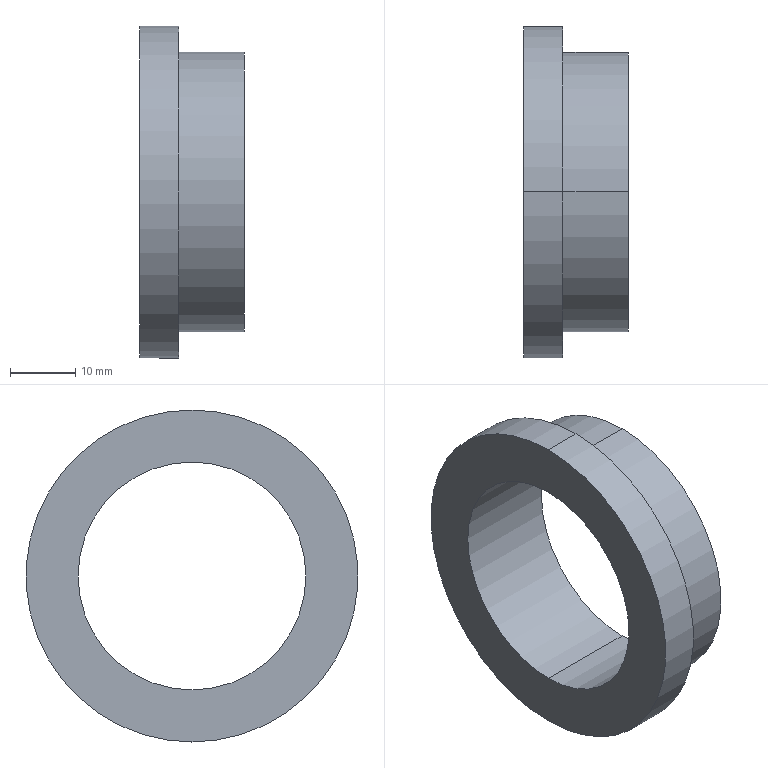Part | SolidWorks | features Revolution 1 | 1 solid | 9 faces | box 16 x 51 x 51 mm | volume 11385 mm3 | cylinder 6 | plane 3 | commonest cylinder face diameters 35 x2 43 x2 51 x2
STEP:
#1=CARTESIAN_POINT('',(-15.343,0.,25.5));
#2=VERTEX_POINT('',#1);
#3=CARTESIAN_POINT('',(-15.343,0.,-25.5));
#4=VERTEX_POINT('',#3);
#5=CARTESIAN_POINT('',(-15.343,0.,0.));
#6=DIRECTION('',(-1.,0.,0.));
#7=DIRECTION('',(0.,0.,1.));
#8=AXIS2_PLACEMENT_3D('',#5,#6,#7);
#9=CIRCLE('',#8,25.5);
#10=EDGE_CURVE('',#2,#4,#9,.T.);
#11=ORIENTED_EDGE('',*,*,#10,.T.);
#12=CARTESIAN_POINT('',(-21.343,0.,-25.5));
#13=VERTEX_POINT('',#12);
#14=CARTESIAN_POINT('',(0.,0.,-25.5));
#15=DIRECTION('',(-1.,0.,0.));
#16=VECTOR('',#15,1000.);
#17=LINE('',#14,#16);
#18=EDGE_CURVE('',#4,#13,#17,.T.);
#19=ORIENTED_EDGE('',*,*,#18,.T.);
#20=CARTESIAN_POINT('',(-21.343,0.,25.5));
#21=VERTEX_POINT('',#20);
#22=CARTESIAN_POINT('',(-21.343,0.,0.));
#23=DIRECTION('',(-1.,0.,0.));
#24=DIRECTION('',(0.,0.,1.));
#25=AXIS2_PLACEMENT_3D('',#22,#23,#24);
#26=CIRCLE('',#25,25.5);
#27=EDGE_CURVE('',#21,#13,#26,.T.);
#28=ORIENTED_EDGE('',*,*,#27,.F.);
#29=CARTESIAN_POINT('',(0.,0.,25.5));
#30=DIRECTION('',(-1.,0.,0.));
#31=VECTOR('',#30,1000.);
#32=LINE('',#29,#31);
#33=EDGE_CURVE('',#2,#21,#32,.T.);
#34=ORIENTED_EDGE('',*,*,#33,.F.);
#35=EDGE_LOOP('',(#11,#19,#28,#34));
#36=FACE_OUTER_BOUND('',#35,.T.);
#37=CARTESIAN_POINT('',(0.,0.,0.));
#38=DIRECTION('',(-1.,0.,0.));
#39=DIRECTION('',(0.,0.,1.));
#40=AXIS2_PLACEMENT_3D('',#37,#38,#39);
#41=CYLINDRICAL_SURFACE('',#40,25.5);
#42=ADVANCED_FACE('',(#36),#41,.T.);
#43=CARTESIAN_POINT('',(-5.343,0.,21.5));
#44=VERTEX_POINT('',#43);
#45=CARTESIAN_POINT('',(-5.343,0.,-21.5));
#46=VERTEX_POINT('',#45);
#47=CARTESIAN_POINT('',(-5.343,0.,0.));
#48=DIRECTION('',(-1.,0.,0.));
#49=DIRECTION('',(0.,0.,1.));
#50=AXIS2_PLACEMENT_3D('',#47,#48,#49);
#51=CIRCLE('',#50,21.5);
#52=EDGE_CURVE('',#44,#46,#51,.T.);
#53=ORIENTED_EDGE('',*,*,#52,.T.);
#54=CARTESIAN_POINT('',(-15.343,0.,-21.5));
#55=VERTEX_POINT('',#54);
#56=CARTESIAN_POINT('',(0.,0.,-21.5));
#57=DIRECTION('',(-1.,0.,0.));
#58=VECTOR('',#57,1000.);
#59=LINE('',#56,#58);
#60=EDGE_CURVE('',#46,#55,#59,.T.);
#61=ORIENTED_EDGE('',*,*,#60,.T.);
#62=CARTESIAN_POINT('',(-15.343,0.,21.5));
#63=VERTEX_POINT('',#62);
#64=CARTESIAN_POINT('',(-15.343,0.,0.));
#65=DIRECTION('',(-1.,0.,0.));
#66=DIRECTION('',(0.,0.,1.));
#67=AXIS2_PLACEMENT_3D('',#64,#65,#66);
#68=CIRCLE('',#67,21.5);
#69=EDGE_CURVE('',#63,#55,#68,.T.);
#70=ORIENTED_EDGE('',*,*,#69,.F.);
#71=CARTESIAN_POINT('',(0.,0.,21.5));
#72=DIRECTION('',(-1.,0.,0.));
#73=VECTOR('',#72,1000.);
#74=LINE('',#71,#73);
#75=EDGE_CURVE('',#44,#63,#74,.T.);
#76=ORIENTED_EDGE('',*,*,#75,.F.);
#77=EDGE_LOOP('',(#53,#61,#70,#76));
#78=FACE_OUTER_BOUND('',#77,.T.);
#79=CARTESIAN_POINT('',(0.,0.,0.));
#80=DIRECTION('',(-1.,0.,0.));
#81=DIRECTION('',(0.,0.,1.));
#82=AXIS2_PLACEMENT_3D('',#79,#80,#81);
#83=CYLINDRICAL_SURFACE('',#82,21.5);
#84=ADVANCED_FACE('',(#78),#83,.T.);
#85=CARTESIAN_POINT('',(-5.343,0.,-17.5));
#86=VERTEX_POINT('',#85);
#87=CARTESIAN_POINT('',(-5.343,0.,17.5));
#88=VERTEX_POINT('',#87);
#89=CARTESIAN_POINT('',(-5.343,0.,0.));
#90=DIRECTION('',(-1.,0.,0.));
#91=DIRECTION('',(0.,0.,1.));
#92=AXIS2_PLACEMENT_3D('',#89,#90,#91);
#93=CIRCLE('',#92,17.5);
#94=EDGE_CURVE('',#86,#88,#93,.T.);
#95=ORIENTED_EDGE('',*,*,#94,.F.);
#96=CARTESIAN_POINT('',(-21.343,0.,-17.5));
#97=VERTEX_POINT('',#96);
#98=CARTESIAN_POINT('',(0.,0.,-17.5));
#99=DIRECTION('',(-1.,0.,0.));
#100=VECTOR('',#99,1000.);
#101=LINE('',#98,#100);
#102=EDGE_CURVE('',#86,#97,#101,.T.);
#103=ORIENTED_EDGE('',*,*,#102,.T.);
#104=CARTESIAN_POINT('',(-21.343,0.,17.5));
#105=VERTEX_POINT('',#104);
#106=CARTESIAN_POINT('',(-21.343,0.,0.));
#107=DIRECTION('',(-1.,0.,0.));
#108=DIRECTION('',(0.,0.,1.));
#109=AXIS2_PLACEMENT_3D('',#106,#107,#108);
#110=CIRCLE('',#109,17.5);
#111=EDGE_CURVE('',#97,#105,#110,.T.);
#112=ORIENTED_EDGE('',*,*,#111,.T.);
#113=CARTESIAN_POINT('',(0.,0.,17.5));
#114=DIRECTION('',(-1.,0.,0.));
#115=VECTOR('',#114,1000.);
#116=LINE('',#113,#115);
#117=EDGE_CURVE('',#88,#105,#116,.T.);
#118=ORIENTED_EDGE('',*,*,#117,.F.);
#119=EDGE_LOOP('',(#95,#103,#112,#118));
#120=FACE_OUTER_BOUND('',#119,.T.);
#121=CARTESIAN_POINT('',(0.,0.,0.));
#122=DIRECTION('',(-1.,0.,0.));
#123=DIRECTION('',(0.,0.,1.));
#124=AXIS2_PLACEMENT_3D('',#121,#122,#123);
#125=CYLINDRICAL_SURFACE('',#124,17.5);
#126=ADVANCED_FACE('',(#120),#125,.F.);
#127=ORIENTED_EDGE('',*,*,#102,.F.);
#128=CARTESIAN_POINT('',(-5.343,0.,0.));
#129=DIRECTION('',(-1.,0.,0.));
#130=DIRECTION('',(0.,0.,1.));
#131=AXIS2_PLACEMENT_3D('',#128,#129,#130);
#132=CIRCLE('',#131,17.5);
#133=EDGE_CURVE('',#88,#86,#132,.T.);
#134=ORIENTED_EDGE('',*,*,#133,.F.);
#135=ORIENTED_EDGE('',*,*,#117,.T.);
#136=CARTESIAN_POINT('',(-21.343,0.,0.));
#137=DIRECTION('',(-1.,0.,0.));
#138=DIRECTION('',(0.,0.,1.));
#139=AXIS2_PLACEMENT_3D('',#136,#137,#138);
#140=CIRCLE('',#139,17.5);
#141=EDGE_CURVE('',#105,#97,#140,.T.);
#142=ORIENTED_EDGE('',*,*,#141,.T.);
#143=EDGE_LOOP('',(#127,#134,#135,#142));
#144=FACE_OUTER_BOUND('',#143,.T.);
#145=CARTESIAN_POINT('',(0.,0.,0.));
#146=DIRECTION('',(-1.,0.,0.));
#147=DIRECTION('',(0.,0.,1.));
#148=AXIS2_PLACEMENT_3D('',#145,#146,#147);
#149=CYLINDRICAL_SURFACE('',#148,17.5);
#150=ADVANCED_FACE('',(#144),#149,.F.);
#151=ORIENTED_EDGE('',*,*,#52,.F.);
#152=CARTESIAN_POINT('',(-5.343,0.,0.));
#153=DIRECTION('',(-1.,0.,0.));
#154=DIRECTION('',(0.,0.,1.));
#155=AXIS2_PLACEMENT_3D('',#152,#153,#154);
#156=CIRCLE('',#155,21.5);
#157=EDGE_CURVE('',#46,#44,#156,.T.);
#158=ORIENTED_EDGE('',*,*,#157,.F.);
#159=EDGE_LOOP('',(#151,#158));
#160=FACE_OUTER_BOUND('',#159,.T.);
#161=ORIENTED_EDGE('',*,*,#133,.T.);
#162=ORIENTED_EDGE('',*,*,#94,.T.);
#163=EDGE_LOOP('',(#161,#162));
#164=FACE_BOUND('',#163,.T.);
#165=CARTESIAN_POINT('',(-5.343,17.5,0.));
#166=DIRECTION('',(-1.,0.,0.));
#167=DIRECTION('',(0.,0.,1.));
#168=AXIS2_PLACEMENT_3D('',#165,#166,#167);
#169=PLANE('',#168);
#170=ADVANCED_FACE('',(#160,#164),#169,.F.);
#171=ORIENTED_EDGE('',*,*,#60,.F.);
#172=ORIENTED_EDGE('',*,*,#157,.T.);
#173=ORIENTED_EDGE('',*,*,#75,.T.);
#174=CARTESIAN_POINT('',(-15.343,0.,0.));
#175=DIRECTION('',(-1.,0.,0.));
#176=DIRECTION('',(0.,0.,1.));
#177=AXIS2_PLACEMENT_3D('',#174,#175,#176);
#178=CIRCLE('',#177,21.5);
#179=EDGE_CURVE('',#55,#63,#178,.T.);
#180=ORIENTED_EDGE('',*,*,#179,.F.);
#181=EDGE_LOOP('',(#171,#172,#173,#180));
#182=FACE_OUTER_BOUND('',#181,.T.);
#183=CARTESIAN_POINT('',(0.,0.,0.));
#184=DIRECTION('',(-1.,0.,0.));
#185=DIRECTION('',(0.,0.,1.));
#186=AXIS2_PLACEMENT_3D('',#183,#184,#185);
#187=CYLINDRICAL_SURFACE('',#186,21.5);
#188=ADVANCED_FACE('',(#182),#187,.T.);
#189=ORIENTED_EDGE('',*,*,#10,.F.);
#190=CARTESIAN_POINT('',(-15.343,0.,0.));
#191=DIRECTION('',(-1.,0.,0.));
#192=DIRECTION('',(0.,0.,1.));
#193=AXIS2_PLACEMENT_3D('',#190,#191,#192);
#194=CIRCLE('',#193,25.5);
#195=EDGE_CURVE('',#4,#2,#194,.T.);
#196=ORIENTED_EDGE('',*,*,#195,.F.);
#197=EDGE_LOOP('',(#189,#196));
#198=FACE_OUTER_BOUND('',#197,.T.);
#199=ORIENTED_EDGE('',*,*,#69,.T.);
#200=ORIENTED_EDGE('',*,*,#179,.T.);
#201=EDGE_LOOP('',(#199,#200));
#202=FACE_BOUND('',#201,.T.);
#203=CARTESIAN_POINT('',(-15.343,21.5,0.));
#204=DIRECTION('',(-1.,0.,0.));
#205=DIRECTION('',(0.,0.,1.));
#206=AXIS2_PLACEMENT_3D('',#203,#204,#205);
#207=PLANE('',#206);
#208=ADVANCED_FACE('',(#198,#202),#207,.F.);
#209=ORIENTED_EDGE('',*,*,#18,.F.);
#210=ORIENTED_EDGE('',*,*,#195,.T.);
#211=ORIENTED_EDGE('',*,*,#33,.T.);
#212=CARTESIAN_POINT('',(-21.343,0.,0.));
#213=DIRECTION('',(-1.,0.,0.));
#214=DIRECTION('',(0.,0.,1.));
#215=AXIS2_PLACEMENT_3D('',#212,#213,#214);
#216=CIRCLE('',#215,25.5);
#217=EDGE_CURVE('',#13,#21,#216,.T.);
#218=ORIENTED_EDGE('',*,*,#217,.F.);
#219=EDGE_LOOP('',(#209,#210,#211,#218));
#220=FACE_OUTER_BOUND('',#219,.T.);
#221=CARTESIAN_POINT('',(0.,0.,0.));
#222=DIRECTION('',(-1.,0.,0.));
#223=DIRECTION('',(0.,0.,1.));
#224=AXIS2_PLACEMENT_3D('',#221,#222,#223);
#225=CYLINDRICAL_SURFACE('',#224,25.5);
#226=ADVANCED_FACE('',(#220),#225,.T.);
#227=ORIENTED_EDGE('',*,*,#141,.F.);
#228=ORIENTED_EDGE('',*,*,#111,.F.);
#229=EDGE_LOOP('',(#227,#228));
#230=FACE_BOUND('',#229,.T.);
#231=ORIENTED_EDGE('',*,*,#27,.T.);
#232=ORIENTED_EDGE('',*,*,#217,.T.);
#233=EDGE_LOOP('',(#231,#232));
#234=FACE_OUTER_BOUND('',#233,.T.);
#235=CARTESIAN_POINT('',(-21.343,25.5,0.));
#236=DIRECTION('',(1.,0.,0.));
#237=DIRECTION('',(0.,0.,-1.));
#238=AXIS2_PLACEMENT_3D('',#235,#236,#237);
#239=PLANE('',#238);
#240=ADVANCED_FACE('',(#230,#234),#239,.F.);
#241=CLOSED_SHELL('',(#42,#84,#126,#150,#170,#188,#208,#226,#240));
#242=MANIFOLD_SOLID_BREP('',#241);
#243=CARTESIAN_POINT('',(0.,0.,0.));
#244=DIRECTION('',(0.,0.,1.));
#245=DIRECTION('',(1.,0.,0.));
#246=AXIS2_PLACEMENT_3D('',#243,#244,#245);
#247=(LENGTH_UNIT()NAMED_UNIT(*)SI_UNIT(.MILLI.,.METRE.));
#248=UNCERTAINTY_MEASURE_WITH_UNIT(LENGTH_MEASURE(0.00001),#247,'','');
#249=(NAMED_UNIT(*)PLANE_ANGLE_UNIT()SI_UNIT($,.RADIAN.));
#250=(NAMED_UNIT(*)SI_UNIT($,.STERADIAN.)SOLID_ANGLE_UNIT());
#251=(GEOMETRIC_REPRESENTATION_CONTEXT(3)GLOBAL_UNCERTAINTY_ASSIGNED_CONTEXT((#248))GLOBAL_UNIT_ASSIGNED_CONTEXT((#247,#249,#250))REPRESENTATION_CONTEXT('',''));
#252=ADVANCED_BREP_SHAPE_REPRESENTATION('',(#242,#246),#251);